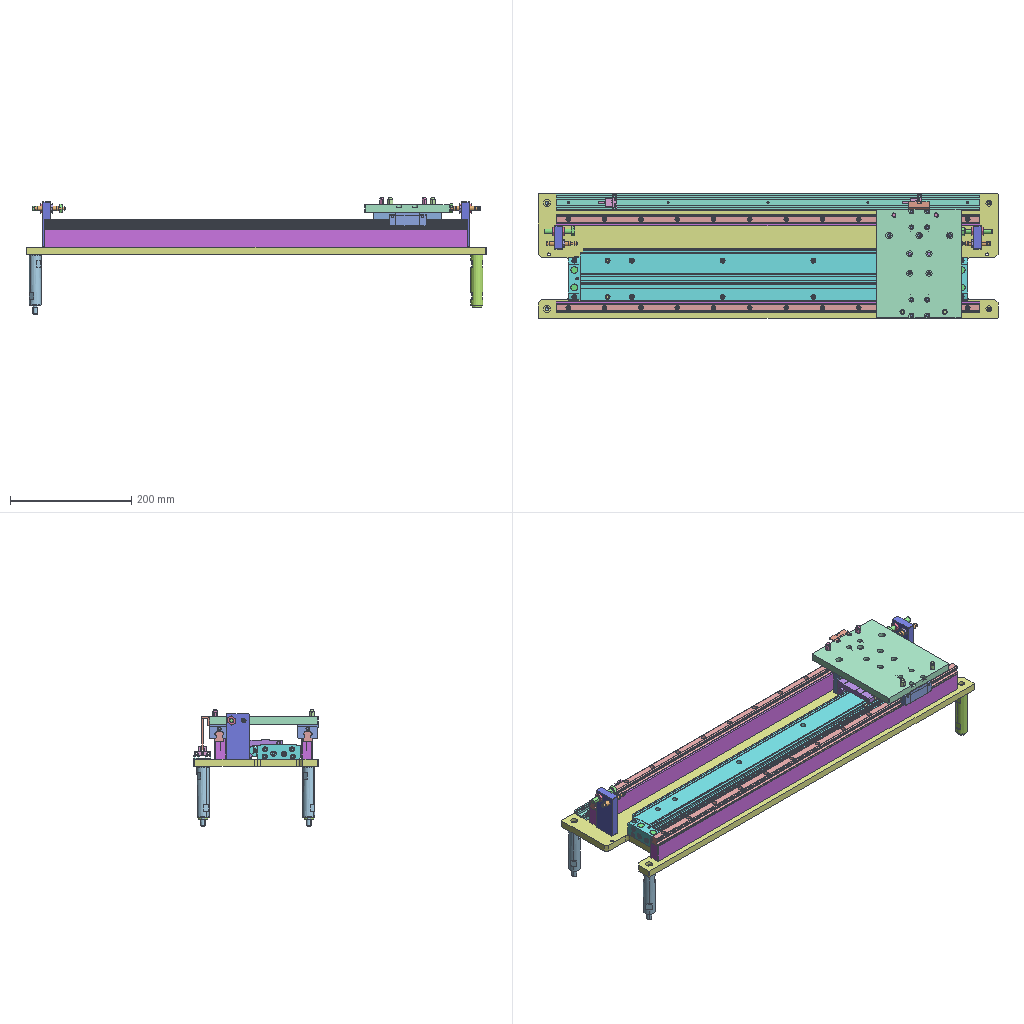Assembly | SolidWorks | 25 different items | 50 placed | box 760 x 205 x 193 mm
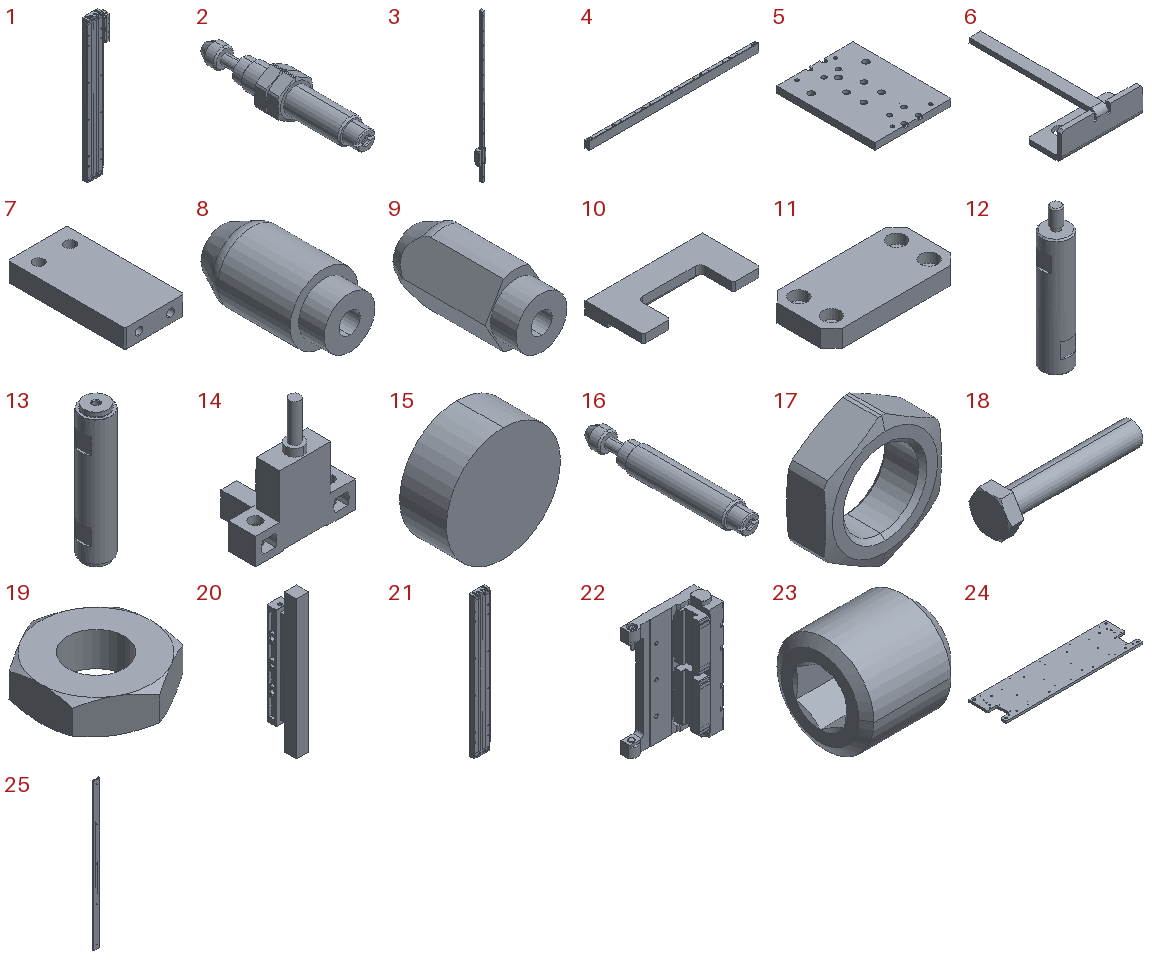Parts list (item | name | quantity | parent item | size | volume | features):
1 | (subassembly) | x1 | - | 105 x 32 x 660 mm | 1112378 mm3 | features AEMSimFeature 1
2 | (subassembly) | x2 | - | 11 x 52 x 12.325 mm | 2543 mm3 | -
3 | (subassembly) | x2 | - | 34 x 28 x 700 mm | 165432 mm3 | -
4 | - | x2 | - | 700 x 18 x 33 mm | 370685 mm3 | features HoleWzd 3, Chamfer 1, Extrusion 1, ICE 1
5 | - | x1 | - | 140 x 180 x 12 mm | 292625 mm3 | features HoleWzd 7, Chamfer 1, Extrusion 1, ICE 1
6 | - | x1 | - | 35 x 55 x 12 mm | 2052 mm3 | features EdgeFlange 2, Chamfer 1, FlatPattern 1, HoleWzd 1, SMBaseFlange 1, SheetMetal 1
7 | - | x2 | - | 38 x 75 x 12 mm | 32833 mm3 | features HoleWzd 3, Chamfer 1, Extrusion 1
8 | - | x2 | - | 8 x 15 x 8 mm | 587.79 mm3 | features Fillet 1, HoleWzd 1, Revolution 1
9 | - | x2 | - | 7.282 x 15 x 8 mm | 482.004 mm3 | features Fillet 1, HoleWzd 1, ICE 1, Revolution 1
10 | - | x1 | - | 112 x 56 x 12 mm | 43333 mm3 | features ICE 2, Chamfer 1, Extrusion 1, Fillet 1, HoleWzd 1
11 | - | x1 | - | 60 x 30 x 8 mm | 12886 mm3 | features Chamfer 1, Extrusion 1, HoleWzd 1
12 | - | x2 | - | 20 x 20 x 99 mm | 26273 mm3 | features BaseBody 1
13 | - | x2 | - | 20 x 20 x 90 mm | 26843 mm3 | features BaseBody 1
14 | - | x2 | - | 26.2 x 15.7 x 30.7 mm | 2541 mm3 | features BaseBody 1
15 | - | x4 | in 1 | 11 x 4.5 x 11 mm | 427.649 mm3 | features BaseBody 1
16 | - | x2 | in 2 | 8 x 52 x 8 mm | 2052 mm3 | features BaseBody 1
17 | - | x4 | in 2 | 11 x 4 x 12.325 mm | 245.478 mm3 | features BaseBody 1
18 | - | x2 | - | 50.3 x 15.011 x 13 mm | 3008 mm3 | features BaseBody 1
19 | - | x4 | - | 13 x 15.011 x 4 mm | 441.798 mm3 | features BaseBody 1
20 | - | x1 | in 1 | 12 x 25 x 120 mm | 23064 mm3 | features BaseBody 1
21 | - | x1 | in 1 | 85.5 x 24 x 660 mm | 981928 mm3 | features BaseBody 1
22 | - | x1 | in 1 | 75 x 30.5 x 119.8 mm | 105188 mm3 | features BaseBody 1
23 | - | x6 | in 1 | 5 x 5 x 5 mm | 82.303 mm3 | features BaseBody 1
24 | - | x1 | - | 760 x 205 x 12 mm | 1773307 mm3 | features HoleWzd 8, Chamfer 2, ICE 2, Extrusion 1, Fillet 1
25 | - | x1 | - | 28 x 6 x 700 mm | 58418 mm3 | features BaseBody 1, HoleWzd 1, ICE 1
Mates (type | each side: item.copy, entity, surface, feature):
Coincident | 24.1 face plane Boss-Extrude1 | 4.1 face plane Boss-Extrude1
Coincident | 24.1 face plane Boss-Extrude1 | 4.2 face plane Boss-Extrude1
Width | 4.2 face plane Boss-Extrude1 | 4.2 face plane Boss-Extrude1 | 24.1 face plane Boss-Extrude1 | 24.1 face plane Boss-Extrude1
Width | 6.1 face plane Base-Flange1 | 6.1 face plane Base-Flange1 | 5.1 face plane Boss-Extrude1 | 5.1 face plane Boss-Extrude1
Coincident | 5.1 face plane Boss-Extrude1 | 6.1 face plane Edge-Flange3
Coincident | 24.1 face plane Boss-Extrude1 | 25.1 face plane Input1 | 2 times
Coincident | 24.1 face plane Boss-Extrude1 | 5.1 face plane Boss-Extrude1
Width | 25.1 face plane Input1 | 25.1 face plane Boss-Extrude1 | 24.1 face plane Boss-Extrude1 | 24.1 face plane Boss-Extrude1
Concentric | 24.1 face cylinder Cut-Extrude1 | 13.1 face cylinder Input1
Coincident | 24.1 face plane Cut-Extrude1 | 13.1 face plane Input1
Concentric | 24.1 face cylinder Cut-Extrude1 | 13.2 face cylinder Input1
Coincident | 24.1 face plane Cut-Extrude1 | 13.2 face plane Input1
Width | 4.1 face plane Boss-Extrude1 | 4.1 face plane Boss-Extrude1 | 24.1 face plane Boss-Extrude1 | 24.1 face plane Boss-Extrude1
Coincident | 25.1 face plane Input1 | 14.1 face plane Input1
Width | 14.1 face plane Input1 | 14.1 face plane Input1 | 25.1 face plane Input1 | 25.1 face plane Input1
Width | 14.1 face plane Input1 | 14.1 face plane Input1 | 6.1 face plane Edge-Flange4 | 6.1 face plane Edge-Flange4
Coincident | 25.1 face plane Input1 | 14.2 face plane Input1
Width | 14.2 face plane Input1 | 14.2 face plane Input1 | 25.1 face plane Input1 | 25.1 face plane Input1
DistanceDim | 14.2 face plane Input1 | 25.1 face plane Boss-Extrude1
Concentric | 7.1 face cylinder M8 Tapped Hole1 | 16.1 face cylinder Input1
Concentric | 7.1 face cylinder M8 Tapped Hole2 | 18.1 face cylinder Input1
Coincident | 7.1 face plane Boss-Extrude1 | 19.1 face plane Input1
Coincident | 7.1 face plane Boss-Extrude1 | 19.2 face plane Input1
DistanceDim | 18.1 face plane Input1 | 16.1 face plane Input1
Concentric | 18.1 face cylinder Input1 | 19.2 face cylinder Input1
Concentric | 18.1 face cylinder Input1 | 19.1 face cylinder Input1
Coincident | 24.1 face plane Boss-Extrude1 | 7.1 face plane Boss-Extrude1
Coincident | 24.1 face plane Boss-Extrude1 | 7.2 face plane Boss-Extrude1
DistanceDim | 16.1 face plane Input1 | 5.1 face plane Boss-Extrude1
DistanceDim | 7.1 face plane Boss-Extrude1 | 24.1 face plane Boss-Extrude1
Concentric | 7.2 face cylinder M8 Tapped Hole1 | 16.2 face cylinder Input1
Concentric | 7.2 face cylinder M8 Tapped Hole2 | 18.2 face cylinder Input1
Concentric | 5.1 face cylinder Size mm dowel hole 2 | 8.1 face cylinder Revolve1
Coincident | 5.1 face plane Size mm dowel hole 2 | 8.1 face plane Revolve1
Concentric | 5.1 face cylinder Size mm dowel hole 2 | 8.2 face cylinder Revolve1
Coincident | 5.1 face plane Size mm dowel hole 2 | 8.2 face plane Revolve1
Concentric | 5.1 face cylinder CBORE for M3 Hex Socket Head Cap Screw1 | 9.1 face cylinder Revolve1
Coincident | 5.1 face plane Size mm dowel hole 2 | 9.1 face plane Revolve1
Concentric | 5.1 face cylinder Size mm dowel hole 2 | 9.2 face cylinder Revolve1
Coincident | 5.1 face plane Size mm dowel hole 2 | 9.2 face plane Revolve1
Coincident | 24.1 face plane Boss-Extrude1 | 12.1 face plane Input1
Concentric | 24.1 face cylinder CBORE for M6 Hex Head Flange Bolt1 | 12.1 face cylinder Input1
Concentric | 24.1 face cylinder CBORE for M6 Hex Head Flange Bolt1 | 12.2 face cylinder Input1
Coincident | 24.1 face plane Boss-Extrude1 | 12.2 face plane Input1
Concentric | 18.2 face cylinder Input1 | 19.3 face cylinder Input1
Coincident | 7.2 face plane Boss-Extrude1 | 19.3 face plane Input1
Coincident | 7.2 face plane Boss-Extrude1 | 19.4 face plane Input1
Concentric | 18.2 face cylinder Input1 | 19.4 face cylinder Input1
Coincident | 24.1 face plane Boss-Extrude1 | 21.1 face plane Input1
Concentric | 24.1 face cylinder M4 Tapped Hole1 | 21.1 face cylinder Input1 | 2 times
Coincident | 5.1 face plane Boss-Extrude1 | 10.1 face plane Boss-Extrude1
Concentric | 5.1 face cylinder CBORE for M6 Hex Socket Head Cap Screw1 | 10.1 face cylinder M6 Tapped Hole1 | 2 times
Coincident | 22.1 face plane Input1 | 11.1 face plane Boss-Extrude1
Concentric | 22.1 face cylinder Input1 | 11.1 face cylinder CBORE for M4 Hex Socket Head Cap Screw1 | 2 times
Coincident | 10.1 face plane Cut-Extrude2 | 11.1 face plane Boss-Extrude1